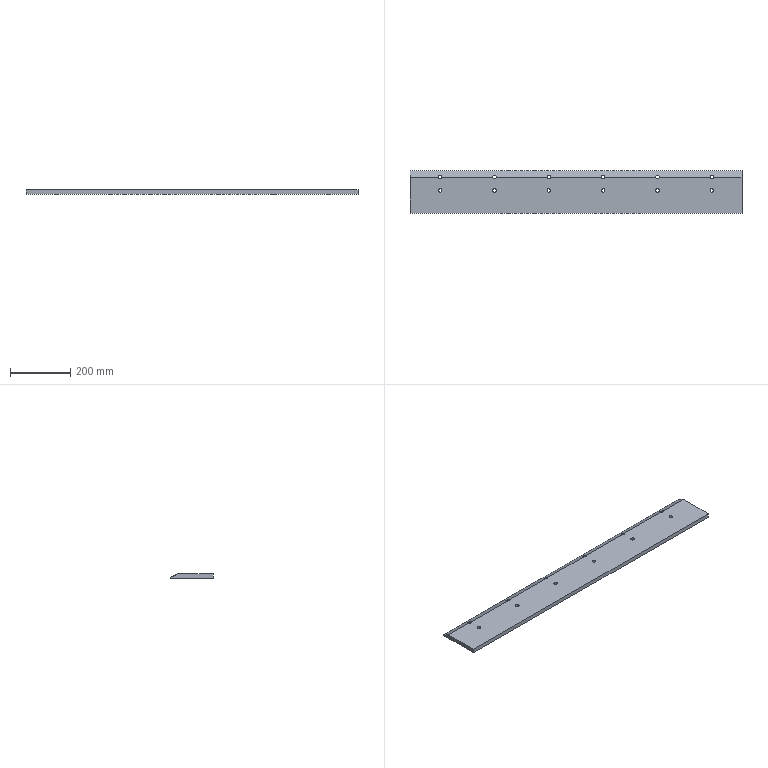Part | SolidWorks | features Chamfer 1, FlatPattern 1, SMBaseFlange 1, SheetMetal 1 | 1 solid | 31 faces | box 1100 x 140 x 14 mm | volume 1986347 mm3 | cylinder 24 | plane 7 | commonest cylinder face diameters 12 x24
STEP:
#1=CARTESIAN_POINT('',(1503.918,1234.342,-14.));
#2=VERTEX_POINT('',#1);
#3=CARTESIAN_POINT('',(1515.918,1234.342,-14.));
#4=VERTEX_POINT('',#3);
#5=CARTESIAN_POINT('',(1509.918,1234.342,-14.));
#6=DIRECTION('',(0.,0.,1.));
#7=DIRECTION('',(1.,0.,0.));
#8=AXIS2_PLACEMENT_3D('',#5,#6,#7);
#9=CIRCLE('',#8,6.);
#10=EDGE_CURVE('',#2,#4,#9,.T.);
#11=ORIENTED_EDGE('',*,*,#10,.F.);
#12=CARTESIAN_POINT('',(1503.918,1234.342,0.));
#13=VERTEX_POINT('',#12);
#14=CARTESIAN_POINT('',(1503.918,1234.342,-14.));
#15=DIRECTION('',(0.,0.,1.));
#16=VECTOR('',#15,1000.);
#17=LINE('',#14,#16);
#18=EDGE_CURVE('',#2,#13,#17,.T.);
#19=ORIENTED_EDGE('',*,*,#18,.T.);
#20=CARTESIAN_POINT('',(1515.918,1234.342,0.));
#21=VERTEX_POINT('',#20);
#22=CARTESIAN_POINT('',(1509.918,1234.342,0.));
#23=DIRECTION('',(0.,0.,1.));
#24=DIRECTION('',(1.,0.,0.));
#25=AXIS2_PLACEMENT_3D('',#22,#23,#24);
#26=CIRCLE('',#25,6.);
#27=EDGE_CURVE('',#13,#21,#26,.T.);
#28=ORIENTED_EDGE('',*,*,#27,.T.);
#29=CARTESIAN_POINT('',(1515.918,1234.342,-14.));
#30=DIRECTION('',(0.,0.,1.));
#31=VECTOR('',#30,1000.);
#32=LINE('',#29,#31);
#33=EDGE_CURVE('',#4,#21,#32,.T.);
#34=ORIENTED_EDGE('',*,*,#33,.F.);
#35=EDGE_LOOP('',(#11,#19,#28,#34));
#36=FACE_OUTER_BOUND('',#35,.T.);
#37=CARTESIAN_POINT('',(1509.918,1234.342,-14.));
#38=DIRECTION('',(0.,0.,1.));
#39=DIRECTION('',(1.,0.,0.));
#40=AXIS2_PLACEMENT_3D('',#37,#38,#39);
#41=CYLINDRICAL_SURFACE('',#40,6.);
#42=ADVANCED_FACE('',(#36),#41,.F.);
#43=CARTESIAN_POINT('',(1683.918,1234.342,-14.));
#44=VERTEX_POINT('',#43);
#45=CARTESIAN_POINT('',(1695.918,1234.342,-14.));
#46=VERTEX_POINT('',#45);
#47=CARTESIAN_POINT('',(1689.918,1234.342,-14.));
#48=DIRECTION('',(0.,0.,1.));
#49=DIRECTION('',(1.,0.,0.));
#50=AXIS2_PLACEMENT_3D('',#47,#48,#49);
#51=CIRCLE('',#50,6.);
#52=EDGE_CURVE('',#44,#46,#51,.T.);
#53=ORIENTED_EDGE('',*,*,#52,.F.);
#54=CARTESIAN_POINT('',(1683.918,1234.342,0.));
#55=VERTEX_POINT('',#54);
#56=CARTESIAN_POINT('',(1683.918,1234.342,-14.));
#57=DIRECTION('',(0.,0.,1.));
#58=VECTOR('',#57,1000.);
#59=LINE('',#56,#58);
#60=EDGE_CURVE('',#44,#55,#59,.T.);
#61=ORIENTED_EDGE('',*,*,#60,.T.);
#62=CARTESIAN_POINT('',(1695.918,1234.342,0.));
#63=VERTEX_POINT('',#62);
#64=CARTESIAN_POINT('',(1689.918,1234.342,0.));
#65=DIRECTION('',(0.,0.,1.));
#66=DIRECTION('',(1.,0.,0.));
#67=AXIS2_PLACEMENT_3D('',#64,#65,#66);
#68=CIRCLE('',#67,6.);
#69=EDGE_CURVE('',#55,#63,#68,.T.);
#70=ORIENTED_EDGE('',*,*,#69,.T.);
#71=CARTESIAN_POINT('',(1695.918,1234.342,-14.));
#72=DIRECTION('',(0.,0.,1.));
#73=VECTOR('',#72,1000.);
#74=LINE('',#71,#73);
#75=EDGE_CURVE('',#46,#63,#74,.T.);
#76=ORIENTED_EDGE('',*,*,#75,.F.);
#77=EDGE_LOOP('',(#53,#61,#70,#76));
#78=FACE_OUTER_BOUND('',#77,.T.);
#79=CARTESIAN_POINT('',(1689.918,1234.342,-14.));
#80=DIRECTION('',(0.,0.,1.));
#81=DIRECTION('',(1.,0.,0.));
#82=AXIS2_PLACEMENT_3D('',#79,#80,#81);
#83=CYLINDRICAL_SURFACE('',#82,6.);
#84=ADVANCED_FACE('',(#78),#83,.F.);
#85=CARTESIAN_POINT('',(1143.918,1234.342,-14.));
#86=VERTEX_POINT('',#85);
#87=CARTESIAN_POINT('',(1155.918,1234.342,-14.));
#88=VERTEX_POINT('',#87);
#89=CARTESIAN_POINT('',(1149.918,1234.342,-14.));
#90=DIRECTION('',(0.,0.,1.));
#91=DIRECTION('',(1.,0.,0.));
#92=AXIS2_PLACEMENT_3D('',#89,#90,#91);
#93=CIRCLE('',#92,6.);
#94=EDGE_CURVE('',#86,#88,#93,.T.);
#95=ORIENTED_EDGE('',*,*,#94,.F.);
#96=CARTESIAN_POINT('',(1143.918,1234.342,0.));
#97=VERTEX_POINT('',#96);
#98=CARTESIAN_POINT('',(1143.918,1234.342,-14.));
#99=DIRECTION('',(0.,0.,1.));
#100=VECTOR('',#99,1000.);
#101=LINE('',#98,#100);
#102=EDGE_CURVE('',#86,#97,#101,.T.);
#103=ORIENTED_EDGE('',*,*,#102,.T.);
#104=CARTESIAN_POINT('',(1155.918,1234.342,0.));
#105=VERTEX_POINT('',#104);
#106=CARTESIAN_POINT('',(1149.918,1234.342,0.));
#107=DIRECTION('',(0.,0.,1.));
#108=DIRECTION('',(1.,0.,0.));
#109=AXIS2_PLACEMENT_3D('',#106,#107,#108);
#110=CIRCLE('',#109,6.);
#111=EDGE_CURVE('',#97,#105,#110,.T.);
#112=ORIENTED_EDGE('',*,*,#111,.T.);
#113=CARTESIAN_POINT('',(1155.918,1234.342,-14.));
#114=DIRECTION('',(0.,0.,1.));
#115=VECTOR('',#114,1000.);
#116=LINE('',#113,#115);
#117=EDGE_CURVE('',#88,#105,#116,.T.);
#118=ORIENTED_EDGE('',*,*,#117,.F.);
#119=EDGE_LOOP('',(#95,#103,#112,#118));
#120=FACE_OUTER_BOUND('',#119,.T.);
#121=CARTESIAN_POINT('',(1149.918,1234.342,-14.));
#122=DIRECTION('',(0.,0.,1.));
#123=DIRECTION('',(1.,0.,0.));
#124=AXIS2_PLACEMENT_3D('',#121,#122,#123);
#125=CYLINDRICAL_SURFACE('',#124,6.);
#126=ADVANCED_FACE('',(#120),#125,.F.);
#127=CARTESIAN_POINT('',(1323.918,1234.342,-14.));
#128=VERTEX_POINT('',#127);
#129=CARTESIAN_POINT('',(1335.918,1234.342,-14.));
#130=VERTEX_POINT('',#129);
#131=CARTESIAN_POINT('',(1329.918,1234.342,-14.));
#132=DIRECTION('',(0.,0.,1.));
#133=DIRECTION('',(1.,0.,0.));
#134=AXIS2_PLACEMENT_3D('',#131,#132,#133);
#135=CIRCLE('',#134,6.);
#136=EDGE_CURVE('',#128,#130,#135,.T.);
#137=ORIENTED_EDGE('',*,*,#136,.F.);
#138=CARTESIAN_POINT('',(1323.918,1234.342,0.));
#139=VERTEX_POINT('',#138);
#140=CARTESIAN_POINT('',(1323.918,1234.342,-14.));
#141=DIRECTION('',(0.,0.,1.));
#142=VECTOR('',#141,1000.);
#143=LINE('',#140,#142);
#144=EDGE_CURVE('',#128,#139,#143,.T.);
#145=ORIENTED_EDGE('',*,*,#144,.T.);
#146=CARTESIAN_POINT('',(1335.918,1234.342,0.));
#147=VERTEX_POINT('',#146);
#148=CARTESIAN_POINT('',(1329.918,1234.342,0.));
#149=DIRECTION('',(0.,0.,1.));
#150=DIRECTION('',(1.,0.,0.));
#151=AXIS2_PLACEMENT_3D('',#148,#149,#150);
#152=CIRCLE('',#151,6.);
#153=EDGE_CURVE('',#139,#147,#152,.T.);
#154=ORIENTED_EDGE('',*,*,#153,.T.);
#155=CARTESIAN_POINT('',(1335.918,1234.342,-14.));
#156=DIRECTION('',(0.,0.,1.));
#157=VECTOR('',#156,1000.);
#158=LINE('',#155,#157);
#159=EDGE_CURVE('',#130,#147,#158,.T.);
#160=ORIENTED_EDGE('',*,*,#159,.F.);
#161=EDGE_LOOP('',(#137,#145,#154,#160));
#162=FACE_OUTER_BOUND('',#161,.T.);
#163=CARTESIAN_POINT('',(1329.918,1234.342,-14.));
#164=DIRECTION('',(0.,0.,1.));
#165=DIRECTION('',(1.,0.,0.));
#166=AXIS2_PLACEMENT_3D('',#163,#164,#165);
#167=CYLINDRICAL_SURFACE('',#166,6.);
#168=ADVANCED_FACE('',(#162),#167,.F.);
#169=CARTESIAN_POINT('',(2043.918,1234.342,-14.));
#170=VERTEX_POINT('',#169);
#171=CARTESIAN_POINT('',(2055.918,1234.342,-14.));
#172=VERTEX_POINT('',#171);
#173=CARTESIAN_POINT('',(2049.918,1234.342,-14.));
#174=DIRECTION('',(0.,0.,1.));
#175=DIRECTION('',(1.,0.,0.));
#176=AXIS2_PLACEMENT_3D('',#173,#174,#175);
#177=CIRCLE('',#176,6.);
#178=EDGE_CURVE('',#170,#172,#177,.T.);
#179=ORIENTED_EDGE('',*,*,#178,.F.);
#180=CARTESIAN_POINT('',(2043.918,1234.342,0.));
#181=VERTEX_POINT('',#180);
#182=CARTESIAN_POINT('',(2043.918,1234.342,-14.));
#183=DIRECTION('',(0.,0.,1.));
#184=VECTOR('',#183,1000.);
#185=LINE('',#182,#184);
#186=EDGE_CURVE('',#170,#181,#185,.T.);
#187=ORIENTED_EDGE('',*,*,#186,.T.);
#188=CARTESIAN_POINT('',(2055.918,1234.342,0.));
#189=VERTEX_POINT('',#188);
#190=CARTESIAN_POINT('',(2049.918,1234.342,0.));
#191=DIRECTION('',(0.,0.,1.));
#192=DIRECTION('',(1.,0.,0.));
#193=AXIS2_PLACEMENT_3D('',#190,#191,#192);
#194=CIRCLE('',#193,6.);
#195=EDGE_CURVE('',#181,#189,#194,.T.);
#196=ORIENTED_EDGE('',*,*,#195,.T.);
#197=CARTESIAN_POINT('',(2055.918,1234.342,-14.));
#198=DIRECTION('',(0.,0.,1.));
#199=VECTOR('',#198,1000.);
#200=LINE('',#197,#199);
#201=EDGE_CURVE('',#172,#189,#200,.T.);
#202=ORIENTED_EDGE('',*,*,#201,.F.);
#203=EDGE_LOOP('',(#179,#187,#196,#202));
#204=FACE_OUTER_BOUND('',#203,.T.);
#205=CARTESIAN_POINT('',(2049.918,1234.342,-14.));
#206=DIRECTION('',(0.,0.,1.));
#207=DIRECTION('',(1.,0.,0.));
#208=AXIS2_PLACEMENT_3D('',#205,#206,#207);
#209=CYLINDRICAL_SURFACE('',#208,6.);
#210=ADVANCED_FACE('',(#204),#209,.F.);
#211=CARTESIAN_POINT('',(1863.918,1234.342,-14.));
#212=VERTEX_POINT('',#211);
#213=CARTESIAN_POINT('',(1875.918,1234.342,-14.));
#214=VERTEX_POINT('',#213);
#215=CARTESIAN_POINT('',(1869.918,1234.342,-14.));
#216=DIRECTION('',(0.,0.,1.));
#217=DIRECTION('',(1.,0.,0.));
#218=AXIS2_PLACEMENT_3D('',#215,#216,#217);
#219=CIRCLE('',#218,6.);
#220=EDGE_CURVE('',#212,#214,#219,.T.);
#221=ORIENTED_EDGE('',*,*,#220,.F.);
#222=CARTESIAN_POINT('',(1863.918,1234.342,0.));
#223=VERTEX_POINT('',#222);
#224=CARTESIAN_POINT('',(1863.918,1234.342,-14.));
#225=DIRECTION('',(0.,0.,1.));
#226=VECTOR('',#225,1000.);
#227=LINE('',#224,#226);
#228=EDGE_CURVE('',#212,#223,#227,.T.);
#229=ORIENTED_EDGE('',*,*,#228,.T.);
#230=CARTESIAN_POINT('',(1875.918,1234.342,0.));
#231=VERTEX_POINT('',#230);
#232=CARTESIAN_POINT('',(1869.918,1234.342,0.));
#233=DIRECTION('',(0.,0.,1.));
#234=DIRECTION('',(1.,0.,0.));
#235=AXIS2_PLACEMENT_3D('',#232,#233,#234);
#236=CIRCLE('',#235,6.);
#237=EDGE_CURVE('',#223,#231,#236,.T.);
#238=ORIENTED_EDGE('',*,*,#237,.T.);
#239=CARTESIAN_POINT('',(1875.918,1234.342,-14.));
#240=DIRECTION('',(0.,0.,1.));
#241=VECTOR('',#240,1000.);
#242=LINE('',#239,#241);
#243=EDGE_CURVE('',#214,#231,#242,.T.);
#244=ORIENTED_EDGE('',*,*,#243,.F.);
#245=EDGE_LOOP('',(#221,#229,#238,#244));
#246=FACE_OUTER_BOUND('',#245,.T.);
#247=CARTESIAN_POINT('',(1869.918,1234.342,-14.));
#248=DIRECTION('',(0.,0.,1.));
#249=DIRECTION('',(1.,0.,0.));
#250=AXIS2_PLACEMENT_3D('',#247,#248,#249);
#251=CYLINDRICAL_SURFACE('',#250,6.);
#252=ADVANCED_FACE('',(#246),#251,.F.);
#253=CARTESIAN_POINT('',(1503.918,1279.342,-14.));
#254=VERTEX_POINT('',#253);
#255=CARTESIAN_POINT('',(1515.918,1279.342,-14.));
#256=VERTEX_POINT('',#255);
#257=CARTESIAN_POINT('',(1509.918,1279.342,-14.));
#258=DIRECTION('',(0.,0.,1.));
#259=DIRECTION('',(1.,0.,0.));
#260=AXIS2_PLACEMENT_3D('',#257,#258,#259);
#261=CIRCLE('',#260,6.);
#262=EDGE_CURVE('',#254,#256,#261,.T.);
#263=ORIENTED_EDGE('',*,*,#262,.F.);
#264=CARTESIAN_POINT('',(1503.918,1279.342,-1.565));
#265=VERTEX_POINT('',#264);
#266=CARTESIAN_POINT('',(1503.918,1279.342,-14.));
#267=DIRECTION('',(0.,0.,1.));
#268=VECTOR('',#267,1000.);
#269=LINE('',#266,#268);
#270=EDGE_CURVE('',#254,#265,#269,.T.);
#271=ORIENTED_EDGE('',*,*,#270,.T.);
#272=CARTESIAN_POINT('',(1504.721,1276.342,0.));
#273=VERTEX_POINT('',#272);
#274=CARTESIAN_POINT('',(1503.918,1279.342,-1.565));
#275=CARTESIAN_POINT('',(1503.918,1278.283,-1.013));
#276=CARTESIAN_POINT('',(1504.192,1277.259,-0.4787));
#277=CARTESIAN_POINT('',(1504.721,1276.342,0.));
#278=(BOUNDED_CURVE()B_SPLINE_CURVE(3,(#274,#275,#276,#277),.UNSPECIFIED.,.F.,.T.)B_SPLINE_CURVE_WITH_KNOTS((4,4),(4.712,5.236),.UNSPECIFIED.)CURVE()GEOMETRIC_REPRESENTATION_ITEM()RATIONAL_B_SPLINE_CURVE((1.,0.9773,0.9773,1.))REPRESENTATION_ITEM(''));
#279=EDGE_CURVE('',#265,#273,#278,.T.);
#280=ORIENTED_EDGE('',*,*,#279,.T.);
#281=CARTESIAN_POINT('',(1515.114,1276.342,0.));
#282=VERTEX_POINT('',#281);
#283=CARTESIAN_POINT('',(1509.918,1279.342,0.));
#284=DIRECTION('',(0.,0.,1.));
#285=DIRECTION('',(1.,0.,0.));
#286=AXIS2_PLACEMENT_3D('',#283,#284,#285);
#287=CIRCLE('',#286,6.);
#288=EDGE_CURVE('',#273,#282,#287,.T.);
#289=ORIENTED_EDGE('',*,*,#288,.T.);
#290=CARTESIAN_POINT('',(1515.918,1279.342,-1.565));
#291=VERTEX_POINT('',#290);
#292=CARTESIAN_POINT('',(1515.114,1276.342,0.));
#293=CARTESIAN_POINT('',(1515.643,1277.259,-0.4787));
#294=CARTESIAN_POINT('',(1515.918,1278.283,-1.013));
#295=CARTESIAN_POINT('',(1515.918,1279.342,-1.565));
#296=(BOUNDED_CURVE()B_SPLINE_CURVE(3,(#292,#293,#294,#295),.UNSPECIFIED.,.F.,.T.)B_SPLINE_CURVE_WITH_KNOTS((4,4),(1.047,1.571),.UNSPECIFIED.)CURVE()GEOMETRIC_REPRESENTATION_ITEM()RATIONAL_B_SPLINE_CURVE((1.,0.9773,0.9773,1.))REPRESENTATION_ITEM(''));
#297=EDGE_CURVE('',#282,#291,#296,.T.);
#298=ORIENTED_EDGE('',*,*,#297,.T.);
#299=CARTESIAN_POINT('',(1515.918,1279.342,-14.));
#300=DIRECTION('',(0.,0.,1.));
#301=VECTOR('',#300,1000.);
#302=LINE('',#299,#301);
#303=EDGE_CURVE('',#256,#291,#302,.T.);
#304=ORIENTED_EDGE('',*,*,#303,.F.);
#305=EDGE_LOOP('',(#263,#271,#280,#289,#298,#304));
#306=FACE_OUTER_BOUND('',#305,.T.);
#307=CARTESIAN_POINT('',(1509.918,1279.342,-14.));
#308=DIRECTION('',(0.,0.,1.));
#309=DIRECTION('',(1.,0.,0.));
#310=AXIS2_PLACEMENT_3D('',#307,#308,#309);
#311=CYLINDRICAL_SURFACE('',#310,6.);
#312=ADVANCED_FACE('',(#306),#311,.F.);
#313=CARTESIAN_POINT('',(1683.918,1279.342,-14.));
#314=VERTEX_POINT('',#313);
#315=CARTESIAN_POINT('',(1695.918,1279.342,-14.));
#316=VERTEX_POINT('',#315);
#317=CARTESIAN_POINT('',(1689.918,1279.342,-14.));
#318=DIRECTION('',(0.,0.,1.));
#319=DIRECTION('',(1.,0.,0.));
#320=AXIS2_PLACEMENT_3D('',#317,#318,#319);
#321=CIRCLE('',#320,6.);
#322=EDGE_CURVE('',#314,#316,#321,.T.);
#323=ORIENTED_EDGE('',*,*,#322,.F.);
#324=CARTESIAN_POINT('',(1683.918,1279.342,-1.565));
#325=VERTEX_POINT('',#324);
#326=CARTESIAN_POINT('',(1683.918,1279.342,-14.));
#327=DIRECTION('',(0.,0.,1.));
#328=VECTOR('',#327,1000.);
#329=LINE('',#326,#328);
#330=EDGE_CURVE('',#314,#325,#329,.T.);
#331=ORIENTED_EDGE('',*,*,#330,.T.);
#332=CARTESIAN_POINT('',(1684.721,1276.342,0.));
#333=VERTEX_POINT('',#332);
#334=CARTESIAN_POINT('',(1683.918,1279.342,-1.565));
#335=CARTESIAN_POINT('',(1683.918,1278.283,-1.013));
#336=CARTESIAN_POINT('',(1684.192,1277.259,-0.4787));
#337=CARTESIAN_POINT('',(1684.721,1276.342,0.));
#338=(BOUNDED_CURVE()B_SPLINE_CURVE(3,(#334,#335,#336,#337),.UNSPECIFIED.,.F.,.T.)B_SPLINE_CURVE_WITH_KNOTS((4,4),(4.712,5.236),.UNSPECIFIED.)CURVE()GEOMETRIC_REPRESENTATION_ITEM()RATIONAL_B_SPLINE_CURVE((1.,0.9773,0.9773,1.))REPRESENTATION_ITEM(''));
#339=EDGE_CURVE('',#325,#333,#338,.T.);
#340=ORIENTED_EDGE('',*,*,#339,.T.);
#341=CARTESIAN_POINT('',(1695.114,1276.342,0.));
#342=VERTEX_POINT('',#341);
#343=CARTESIAN_POINT('',(1689.918,1279.342,0.));
#344=DIRECTION('',(0.,0.,1.));
#345=DIRECTION('',(1.,0.,0.));
#346=AXIS2_PLACEMENT_3D('',#343,#344,#345);
#347=CIRCLE('',#346,6.);
#348=EDGE_CURVE('',#333,#342,#347,.T.);
#349=ORIENTED_EDGE('',*,*,#348,.T.);
#350=CARTESIAN_POINT('',(1695.918,1279.342,-1.565));
#351=VERTEX_POINT('',#350);
#352=CARTESIAN_POINT('',(1695.114,1276.342,0.));
#353=CARTESIAN_POINT('',(1695.643,1277.259,-0.4787));
#354=CARTESIAN_POINT('',(1695.918,1278.283,-1.013));
#355=CARTESIAN_POINT('',(1695.918,1279.342,-1.565));
#356=(BOUNDED_CURVE()B_SPLINE_CURVE(3,(#352,#353,#354,#355),.UNSPECIFIED.,.F.,.T.)B_SPLINE_CURVE_WITH_KNOTS((4,4),(1.047,1.571),.UNSPECIFIED.)CURVE()GEOMETRIC_REPRESENTATION_ITEM()RATIONAL_B_SPLINE_CURVE((1.,0.9773,0.9773,1.))REPRESENTATION_ITEM(''));
#357=EDGE_CURVE('',#342,#351,#356,.T.);
#358=ORIENTED_EDGE('',*,*,#357,.T.);
#359=CARTESIAN_POINT('',(1695.918,1279.342,-14.));
#360=DIRECTION('',(0.,0.,1.));
#361=VECTOR('',#360,1000.);
#362=LINE('',#359,#361);
#363=EDGE_CURVE('',#316,#351,#362,.T.);
#364=ORIENTED_EDGE('',*,*,#363,.F.);
#365=EDGE_LOOP('',(#323,#331,#340,#349,#358,#364));
#366=FACE_OUTER_BOUND('',#365,.T.);
#367=CARTESIAN_POINT('',(1689.918,1279.342,-14.));
#368=DIRECTION('',(0.,0.,1.));
#369=DIRECTION('',(1.,0.,0.));
#370=AXIS2_PLACEMENT_3D('',#367,#368,#369);
#371=CYLINDRICAL_SURFACE('',#370,6.);
#372=ADVANCED_FACE('',(#366),#371,.F.);
#373=CARTESIAN_POINT('',(1143.918,1279.342,-14.));
#374=VERTEX_POINT('',#373);
#375=CARTESIAN_POINT('',(1155.918,1279.342,-14.));
#376=VERTEX_POINT('',#375);
#377=CARTESIAN_POINT('',(1149.918,1279.342,-14.));
#378=DIRECTION('',(0.,0.,1.));
#379=DIRECTION('',(1.,0.,0.));
#380=AXIS2_PLACEMENT_3D('',#377,#378,#379);
#381=CIRCLE('',#380,6.);
#382=EDGE_CURVE('',#374,#376,#381,.T.);
#383=ORIENTED_EDGE('',*,*,#382,.F.);
#384=CARTESIAN_POINT('',(1143.918,1279.342,-1.565));
#385=VERTEX_POINT('',#384);
#386=CARTESIAN_POINT('',(1143.918,1279.342,-14.));
#387=DIRECTION('',(0.,0.,1.));
#388=VECTOR('',#387,1000.);
#389=LINE('',#386,#388);
#390=EDGE_CURVE('',#374,#385,#389,.T.);
#391=ORIENTED_EDGE('',*,*,#390,.T.);
#392=CARTESIAN_POINT('',(1144.721,1276.342,0.));
#393=VERTEX_POINT('',#392);
#394=CARTESIAN_POINT('',(1143.918,1279.342,-1.565));
#395=CARTESIAN_POINT('',(1143.918,1278.283,-1.013));
#396=CARTESIAN_POINT('',(1144.192,1277.259,-0.4787));
#397=CARTESIAN_POINT('',(1144.721,1276.342,0.));
#398=(BOUNDED_CURVE()B_SPLINE_CURVE(3,(#394,#395,#396,#397),.UNSPECIFIED.,.F.,.T.)B_SPLINE_CURVE_WITH_KNOTS((4,4),(4.712,5.236),.UNSPECIFIED.)CURVE()GEOMETRIC_REPRESENTATION_ITEM()RATIONAL_B_SPLINE_CURVE((1.,0.9773,0.9773,1.))REPRESENTATION_ITEM(''));
#399=EDGE_CURVE('',#385,#393,#398,.T.);
#400=ORIENTED_EDGE('',*,*,#399,.T.);
#401=CARTESIAN_POINT('',(1155.114,1276.342,0.));
#402=VERTEX_POINT('',#401);
#403=CARTESIAN_POINT('',(1149.918,1279.342,0.));
#404=DIRECTION('',(0.,0.,1.));
#405=DIRECTION('',(1.,0.,0.));
#406=AXIS2_PLACEMENT_3D('',#403,#404,#405);
#407=CIRCLE('',#406,6.);
#408=EDGE_CURVE('',#393,#402,#407,.T.);
#409=ORIENTED_EDGE('',*,*,#408,.T.);
#410=CARTESIAN_POINT('',(1155.918,1279.342,-1.565));
#411=VERTEX_POINT('',#410);
#412=CARTESIAN_POINT('',(1155.114,1276.342,0.));
#413=CARTESIAN_POINT('',(1155.643,1277.259,-0.4787));
#414=CARTESIAN_POINT('',(1155.918,1278.283,-1.013));
#415=CARTESIAN_POINT('',(1155.918,1279.342,-1.565));
#416=(BOUNDED_CURVE()B_SPLINE_CURVE(3,(#412,#413,#414,#415),.UNSPECIFIED.,.F.,.F.)B_SPLINE_CURVE_WITH_KNOTS((4,4),(1.047,1.571),.UNSPECIFIED.)CURVE()GEOMETRIC_REPRESENTATION_ITEM()RATIONAL_B_SPLINE_CURVE((1.,0.9773,0.9773,1.))REPRESENTATION_ITEM(''));
#417=EDGE_CURVE('',#402,#411,#416,.T.);
#418=ORIENTED_EDGE('',*,*,#417,.T.);
#419=CARTESIAN_POINT('',(1155.918,1279.342,-14.));
#420=DIRECTION('',(0.,0.,1.));
#421=VECTOR('',#420,1000.);
#422=LINE('',#419,#421);
#423=EDGE_CURVE('',#376,#411,#422,.T.);
#424=ORIENTED_EDGE('',*,*,#423,.F.);
#425=EDGE_LOOP('',(#383,#391,#400,#409,#418,#424));
#426=FACE_OUTER_BOUND('',#425,.T.);
#427=CARTESIAN_POINT('',(1149.918,1279.342,-14.));
#428=DIRECTION('',(0.,0.,1.));
#429=DIRECTION('',(1.,0.,0.));
#430=AXIS2_PLACEMENT_3D('',#427,#428,#429);
#431=CYLINDRICAL_SURFACE('',#430,6.);
#432=ADVANCED_FACE('',(#426),#431,.F.);
#433=CARTESIAN_POINT('',(1323.918,1279.342,-14.));
#434=VERTEX_POINT('',#433);
#435=CARTESIAN_POINT('',(1335.918,1279.342,-14.));
#436=VERTEX_POINT('',#435);
#437=CARTESIAN_POINT('',(1329.918,1279.342,-14.));
#438=DIRECTION('',(0.,0.,1.));
#439=DIRECTION('',(1.,0.,0.));
#440=AXIS2_PLACEMENT_3D('',#437,#438,#439);
#441=CIRCLE('',#440,6.);
#442=EDGE_CURVE('',#434,#436,#441,.T.);
#443=ORIENTED_EDGE('',*,*,#442,.F.);
#444=CARTESIAN_POINT('',(1323.918,1279.342,-1.565));
#445=VERTEX_POINT('',#444);
#446=CARTESIAN_POINT('',(1323.918,1279.342,-14.));
#447=DIRECTION('',(0.,0.,1.));
#448=VECTOR('',#447,1000.);
#449=LINE('',#446,#448);
#450=EDGE_CURVE('',#434,#445,#449,.T.);
#451=ORIENTED_EDGE('',*,*,#450,.T.);
#452=CARTESIAN_POINT('',(1324.721,1276.342,0.));
#453=VERTEX_POINT('',#452);
#454=CARTESIAN_POINT('',(1323.918,1279.342,-1.565));
#455=CARTESIAN_POINT('',(1323.918,1278.283,-1.013));
#456=CARTESIAN_POINT('',(1324.192,1277.259,-0.4787));
#457=CARTESIAN_POINT('',(1324.721,1276.342,0.));
#458=(BOUNDED_CURVE()B_SPLINE_CURVE(3,(#454,#455,#456,#457),.UNSPECIFIED.,.F.,.T.)B_SPLINE_CURVE_WITH_KNOTS((4,4),(4.712,5.236),.UNSPECIFIED.)CURVE()GEOMETRIC_REPRESENTATION_ITEM()RATIONAL_B_SPLINE_CURVE((1.,0.9773,0.9773,1.))REPRESENTATION_ITEM(''));
#459=EDGE_CURVE('',#445,#453,#458,.T.);
#460=ORIENTED_EDGE('',*,*,#459,.T.);
#461=CARTESIAN_POINT('',(1335.114,1276.342,0.));
#462=VERTEX_POINT('',#461);
#463=CARTESIAN_POINT('',(1329.918,1279.342,0.));
#464=DIRECTION('',(0.,0.,1.));
#465=DIRECTION('',(1.,0.,0.));
#466=AXIS2_PLACEMENT_3D('',#463,#464,#465);
#467=CIRCLE('',#466,6.);
#468=EDGE_CURVE('',#453,#462,#467,.T.);
#469=ORIENTED_EDGE('',*,*,#468,.T.);
#470=CARTESIAN_POINT('',(1335.918,1279.342,-1.565));
#471=VERTEX_POINT('',#470);
#472=CARTESIAN_POINT('',(1335.114,1276.342,0.));
#473=CARTESIAN_POINT('',(1335.643,1277.259,-0.4787));
#474=CARTESIAN_POINT('',(1335.918,1278.283,-1.013));
#475=CARTESIAN_POINT('',(1335.918,1279.342,-1.565));
#476=(BOUNDED_CURVE()B_SPLINE_CURVE(3,(#472,#473,#474,#475),.UNSPECIFIED.,.F.,.F.)B_SPLINE_CURVE_WITH_KNOTS((4,4),(1.047,1.571),.UNSPECIFIED.)CURVE()GEOMETRIC_REPRESENTATION_ITEM()RATIONAL_B_SPLINE_CURVE((1.,0.9773,0.9773,1.))REPRESENTATION_ITEM(''));
#477=EDGE_CURVE('',#462,#471,#476,.T.);
#478=ORIENTED_EDGE('',*,*,#477,.T.);
#479=CARTESIAN_POINT('',(1335.918,1279.342,-14.));
#480=DIRECTION('',(0.,0.,1.));
#481=VECTOR('',#480,1000.);
#482=LINE('',#479,#481);
#483=EDGE_CURVE('',#436,#471,#482,.T.);
#484=ORIENTED_EDGE('',*,*,#483,.F.);
#485=EDGE_LOOP('',(#443,#451,#460,#469,#478,#484));
#486=FACE_OUTER_BOUND('',#485,.T.);
#487=CARTESIAN_POINT('',(1329.918,1279.342,-14.));
#488=DIRECTION('',(0.,0.,1.));
#489=DIRECTION('',(1.,0.,0.));
#490=AXIS2_PLACEMENT_3D('',#487,#488,#489);
#491=CYLINDRICAL_SURFACE('',#490,6.);
#492=ADVANCED_FACE('',(#486),#491,.F.);
#493=CARTESIAN_POINT('',(2043.918,1279.342,-14.));
#494=VERTEX_POINT('',#493);
#495=CARTESIAN_POINT('',(2055.918,1279.342,-14.));
#496=VERTEX_POINT('',#495);
#497=CARTESIAN_POINT('',(2049.918,1279.342,-14.));
#498=DIRECTION('',(0.,0.,1.));
#499=DIRECTION('',(1.,0.,0.));
#500=AXIS2_PLACEMENT_3D('',#497,#498,#499);
#501=CIRCLE('',#500,6.);
#502=EDGE_CURVE('',#494,#496,#501,.T.);
#503=ORIENTED_EDGE('',*,*,#502,.F.);
#504=CARTESIAN_POINT('',(2043.918,1279.342,-1.565));
#505=VERTEX_POINT('',#504);
#506=CARTESIAN_POINT('',(2043.918,1279.342,-14.));
#507=DIRECTION('',(0.,0.,1.));
#508=VECTOR('',#507,1000.);
#509=LINE('',#506,#508);
#510=EDGE_CURVE('',#494,#505,#509,.T.);
#511=ORIENTED_EDGE('',*,*,#510,.T.);
#512=CARTESIAN_POINT('',(2044.721,1276.342,0.));
#513=VERTEX_POINT('',#512);
#514=CARTESIAN_POINT('',(2043.918,1279.342,-1.565));
#515=CARTESIAN_POINT('',(2043.918,1278.283,-1.013));
#516=CARTESIAN_POINT('',(2044.192,1277.259,-0.4787));
#517=CARTESIAN_POINT('',(2044.721,1276.342,0.));
#518=(BOUNDED_CURVE()B_SPLINE_CURVE(3,(#514,#515,#516,#517),.UNSPECIFIED.,.F.,.T.)B_SPLINE_CURVE_WITH_KNOTS((4,4),(4.712,5.236),.UNSPECIFIED.)CURVE()GEOMETRIC_REPRESENTATION_ITEM()RATIONAL_B_SPLINE_CURVE((1.,0.9773,0.9773,1.))REPRESENTATION_ITEM(''));
#519=EDGE_CURVE('',#505,#513,#518,.T.);
#520=ORIENTED_EDGE('',*,*,#519,.T.);
#521=CARTESIAN_POINT('',(2055.114,1276.342,0.));
#522=VERTEX_POINT('',#521);
#523=CARTESIAN_POINT('',(2049.918,1279.342,0.));
#524=DIRECTION('',(0.,0.,1.));
#525=DIRECTION('',(1.,0.,0.));
#526=AXIS2_PLACEMENT_3D('',#523,#524,#525);
#527=CIRCLE('',#526,6.);
#528=EDGE_CURVE('',#513,#522,#527,.T.);
#529=ORIENTED_EDGE('',*,*,#528,.T.);
#530=CARTESIAN_POINT('',(2055.918,1279.342,-1.565));
#531=VERTEX_POINT('',#530);
#532=CARTESIAN_POINT('',(2055.114,1276.342,0.));
#533=CARTESIAN_POINT('',(2055.643,1277.259,-0.4787));
#534=CARTESIAN_POINT('',(2055.918,1278.283,-1.013));
#535=CARTESIAN_POINT('',(2055.918,1279.342,-1.565));
#536=(BOUNDED_CURVE()B_SPLINE_CURVE(3,(#532,#533,#534,#535),.UNSPECIFIED.,.F.,.T.)B_SPLINE_CURVE_WITH_KNOTS((4,4),(1.047,1.571),.UNSPECIFIED.)CURVE()GEOMETRIC_REPRESENTATION_ITEM()RATIONAL_B_SPLINE_CURVE((1.,0.9773,0.9773,1.))REPRESENTATION_ITEM(''));
#537=EDGE_CURVE('',#522,#531,#536,.T.);
#538=ORIENTED_EDGE('',*,*,#537,.T.);
#539=CARTESIAN_POINT('',(2055.918,1279.342,-14.));
#540=DIRECTION('',(0.,0.,1.));
#541=VECTOR('',#540,1000.);
#542=LINE('',#539,#541);
#543=EDGE_CURVE('',#496,#531,#542,.T.);
#544=ORIENTED_EDGE('',*,*,#543,.F.);
#545=EDGE_LOOP('',(#503,#511,#520,#529,#538,#544));
#546=FACE_OUTER_BOUND('',#545,.T.);
#547=CARTESIAN_POINT('',(2049.918,1279.342,-14.));
#548=DIRECTION('',(0.,0.,1.));
#549=DIRECTION('',(1.,0.,0.));
#550=AXIS2_PLACEMENT_3D('',#547,#548,#549);
#551=CYLINDRICAL_SURFACE('',#550,6.);
#552=ADVANCED_FACE('',(#546),#551,.F.);
#553=CARTESIAN_POINT('',(1863.918,1279.342,-14.));
#554=VERTEX_POINT('',#553);
#555=CARTESIAN_POINT('',(1875.918,1279.342,-14.));
#556=VERTEX_POINT('',#555);
#557=CARTESIAN_POINT('',(1869.918,1279.342,-14.));
#558=DIRECTION('',(0.,0.,1.));
#559=DIRECTION('',(1.,0.,0.));
#560=AXIS2_PLACEMENT_3D('',#557,#558,#559);
#561=CIRCLE('',#560,6.);
#562=EDGE_CURVE('',#554,#556,#561,.T.);
#563=ORIENTED_EDGE('',*,*,#562,.F.);
#564=CARTESIAN_POINT('',(1863.918,1279.342,-1.565));
#565=VERTEX_POINT('',#564);
#566=CARTESIAN_POINT('',(1863.918,1279.342,-14.));
#567=DIRECTION('',(0.,0.,1.));
#568=VECTOR('',#567,1000.);
#569=LINE('',#566,#568);
#570=EDGE_CURVE('',#554,#565,#569,.T.);
#571=ORIENTED_EDGE('',*,*,#570,.T.);
#572=CARTESIAN_POINT('',(1864.721,1276.342,0.));
#573=VERTEX_POINT('',#572);
#574=CARTESIAN_POINT('',(1863.918,1279.342,-1.565));
#575=CARTESIAN_POINT('',(1863.918,1278.283,-1.013));
#576=CARTESIAN_POINT('',(1864.192,1277.259,-0.4787));
#577=CARTESIAN_POINT('',(1864.721,1276.342,0.));
#578=(BOUNDED_CURVE()B_SPLINE_CURVE(3,(#574,#575,#576,#577),.UNSPECIFIED.,.F.,.T.)B_SPLINE_CURVE_WITH_KNOTS((4,4),(4.712,5.236),.UNSPECIFIED.)CURVE()GEOMETRIC_REPRESENTATION_ITEM()RATIONAL_B_SPLINE_CURVE((1.,0.9773,0.9773,1.))REPRESENTATION_ITEM(''));
#579=EDGE_CURVE('',#565,#573,#578,.T.);
#580=ORIENTED_EDGE('',*,*,#579,.T.);
#581=CARTESIAN_POINT('',(1875.114,1276.342,0.));
#582=VERTEX_POINT('',#581);
#583=CARTESIAN_POINT('',(1869.918,1279.342,0.));
#584=DIRECTION('',(0.,0.,1.));
#585=DIRECTION('',(1.,0.,0.));
#586=AXIS2_PLACEMENT_3D('',#583,#584,#585);
#587=CIRCLE('',#586,6.);
#588=EDGE_CURVE('',#573,#582,#587,.T.);
#589=ORIENTED_EDGE('',*,*,#588,.T.);
#590=CARTESIAN_POINT('',(1875.918,1279.342,-1.565));
#591=VERTEX_POINT('',#590);
#592=CARTESIAN_POINT('',(1875.114,1276.342,0.));
#593=CARTESIAN_POINT('',(1875.643,1277.259,-0.4787));
#594=CARTESIAN_POINT('',(1875.918,1278.283,-1.013));
#595=CARTESIAN_POINT('',(1875.918,1279.342,-1.565));
#596=(BOUNDED_CURVE()B_SPLINE_CURVE(3,(#592,#593,#594,#595),.UNSPECIFIED.,.F.,.F.)B_SPLINE_CURVE_WITH_KNOTS((4,4),(1.047,1.571),.UNSPECIFIED.)CURVE()GEOMETRIC_REPRESENTATION_ITEM()RATIONAL_B_SPLINE_CURVE((1.,0.9773,0.9773,1.))REPRESENTATION_ITEM(''));
#597=EDGE_CURVE('',#582,#591,#596,.T.);
#598=ORIENTED_EDGE('',*,*,#597,.T.);
#599=CARTESIAN_POINT('',(1875.918,1279.342,-14.));
#600=DIRECTION('',(0.,0.,1.));
#601=VECTOR('',#600,1000.);
#602=LINE('',#599,#601);
#603=EDGE_CURVE('',#556,#591,#602,.T.);
#604=ORIENTED_EDGE('',*,*,#603,.F.);
#605=EDGE_LOOP('',(#563,#571,#580,#589,#598,#604));
#606=FACE_OUTER_BOUND('',#605,.T.);
#607=CARTESIAN_POINT('',(1869.918,1279.342,-14.));
#608=DIRECTION('',(0.,0.,1.));
#609=DIRECTION('',(1.,0.,0.));
#610=AXIS2_PLACEMENT_3D('',#607,#608,#609);
#611=CYLINDRICAL_SURFACE('',#610,6.);
#612=ADVANCED_FACE('',(#606),#611,.F.);
#613=CARTESIAN_POINT('',(1049.918,1299.342,-14.));
#614=VERTEX_POINT('',#613);
#615=CARTESIAN_POINT('',(1049.918,1299.342,-12.));
#616=VERTEX_POINT('',#615);
#617=CARTESIAN_POINT('',(1049.918,1299.342,-14.));
#618=DIRECTION('',(0.,0.,1.));
#619=VECTOR('',#618,1000.);
#620=LINE('',#617,#619);
#621=EDGE_CURVE('',#614,#616,#620,.T.);
#622=ORIENTED_EDGE('',*,*,#621,.T.);
#623=CARTESIAN_POINT('',(2149.918,1299.342,-12.));
#624=VERTEX_POINT('',#623);
#625=CARTESIAN_POINT('',(2149.918,1299.342,-12.));
#626=DIRECTION('',(1.,0.,0.));
#627=VECTOR('',#626,1000.);
#628=LINE('',#625,#627);
#629=EDGE_CURVE('',#616,#624,#628,.T.);
#630=ORIENTED_EDGE('',*,*,#629,.T.);
#631=CARTESIAN_POINT('',(2149.918,1299.342,-14.));
#632=VERTEX_POINT('',#631);
#633=CARTESIAN_POINT('',(2149.918,1299.342,-14.));
#634=DIRECTION('',(0.,0.,1.));
#635=VECTOR('',#634,1000.);
#636=LINE('',#633,#635);
#637=EDGE_CURVE('',#632,#624,#636,.T.);
#638=ORIENTED_EDGE('',*,*,#637,.F.);
#639=CARTESIAN_POINT('',(2149.918,1299.342,-14.));
#640=DIRECTION('',(-1.,0.,0.));
#641=VECTOR('',#640,1000.);
#642=LINE('',#639,#641);
#643=EDGE_CURVE('',#632,#614,#642,.T.);
#644=ORIENTED_EDGE('',*,*,#643,.T.);
#645=EDGE_LOOP('',(#622,#630,#638,#644));
#646=FACE_OUTER_BOUND('',#645,.T.);
#647=CARTESIAN_POINT('',(2149.918,1299.342,-14.));
#648=DIRECTION('',(0.,1.,0.));
#649=DIRECTION('',(-1.,0.,0.));
#650=AXIS2_PLACEMENT_3D('',#647,#648,#649);
#651=PLANE('',#650);
#652=ADVANCED_FACE('',(#646),#651,.T.);
#653=ORIENTED_EDGE('',*,*,#637,.T.);
#654=CARTESIAN_POINT('',(2149.918,1276.342,0.));
#655=VERTEX_POINT('',#654);
#656=CARTESIAN_POINT('',(2149.918,1190.118,44.987));
#657=DIRECTION('',(0.,-0.8866,0.4626));
#658=VECTOR('',#657,1000.);
#659=LINE('',#656,#658);
#660=EDGE_CURVE('',#624,#655,#659,.T.);
#661=ORIENTED_EDGE('',*,*,#660,.T.);
#662=CARTESIAN_POINT('',(2149.918,1159.342,0.));
#663=VERTEX_POINT('',#662);
#664=CARTESIAN_POINT('',(2149.918,1159.342,0.));
#665=DIRECTION('',(0.,1.,0.));
#666=VECTOR('',#665,1000.);
#667=LINE('',#664,#666);
#668=EDGE_CURVE('',#663,#655,#667,.T.);
#669=ORIENTED_EDGE('',*,*,#668,.F.);
#670=CARTESIAN_POINT('',(2149.918,1159.342,-14.));
#671=VERTEX_POINT('',#670);
#672=CARTESIAN_POINT('',(2149.918,1159.342,-14.));
#673=DIRECTION('',(0.,0.,1.));
#674=VECTOR('',#673,1000.);
#675=LINE('',#672,#674);
#676=EDGE_CURVE('',#671,#663,#675,.T.);
#677=ORIENTED_EDGE('',*,*,#676,.F.);
#678=CARTESIAN_POINT('',(2149.918,1159.342,-14.));
#679=DIRECTION('',(0.,1.,0.));
#680=VECTOR('',#679,1000.);
#681=LINE('',#678,#680);
#682=EDGE_CURVE('',#671,#632,#681,.T.);
#683=ORIENTED_EDGE('',*,*,#682,.T.);
#684=EDGE_LOOP('',(#653,#661,#669,#677,#683));
#685=FACE_OUTER_BOUND('',#684,.T.);
#686=CARTESIAN_POINT('',(2149.918,1159.342,-14.));
#687=DIRECTION('',(1.,0.,0.));
#688=DIRECTION('',(0.,0.,-1.));
#689=AXIS2_PLACEMENT_3D('',#686,#687,#688);
#690=PLANE('',#689);
#691=ADVANCED_FACE('',(#685),#690,.T.);
#692=CARTESIAN_POINT('',(1049.918,1159.342,0.));
#693=VERTEX_POINT('',#692);
#694=CARTESIAN_POINT('',(1049.918,1159.342,0.));
#695=DIRECTION('',(1.,0.,0.));
#696=VECTOR('',#695,1000.);
#697=LINE('',#694,#696);
#698=EDGE_CURVE('',#693,#663,#697,.T.);
#699=ORIENTED_EDGE('',*,*,#698,.F.);
#700=CARTESIAN_POINT('',(1049.918,1159.342,-14.));
#701=VERTEX_POINT('',#700);
#702=CARTESIAN_POINT('',(1049.918,1159.342,-14.));
#703=DIRECTION('',(0.,0.,1.));
#704=VECTOR('',#703,1000.);
#705=LINE('',#702,#704);
#706=EDGE_CURVE('',#701,#693,#705,.T.);
#707=ORIENTED_EDGE('',*,*,#706,.F.);
#708=CARTESIAN_POINT('',(1049.918,1159.342,-14.));
#709=DIRECTION('',(1.,0.,0.));
#710=VECTOR('',#709,1000.);
#711=LINE('',#708,#710);
#712=EDGE_CURVE('',#701,#671,#711,.T.);
#713=ORIENTED_EDGE('',*,*,#712,.T.);
#714=ORIENTED_EDGE('',*,*,#676,.T.);
#715=EDGE_LOOP('',(#699,#707,#713,#714));
#716=FACE_OUTER_BOUND('',#715,.T.);
#717=CARTESIAN_POINT('',(1049.918,1159.342,-14.));
#718=DIRECTION('',(0.,-1.,0.));
#719=DIRECTION('',(0.,0.,-1.));
#720=AXIS2_PLACEMENT_3D('',#717,#718,#719);
#721=PLANE('',#720);
#722=ADVANCED_FACE('',(#716),#721,.T.);
#723=CARTESIAN_POINT('',(1049.918,1276.342,0.));
#724=VERTEX_POINT('',#723);
#725=CARTESIAN_POINT('',(1049.918,1299.342,0.));
#726=DIRECTION('',(0.,-1.,0.));
#727=VECTOR('',#726,1000.);
#728=LINE('',#725,#727);
#729=EDGE_CURVE('',#724,#693,#728,.T.);
#730=ORIENTED_EDGE('',*,*,#729,.F.);
#731=CARTESIAN_POINT('',(1049.918,1300.162,-12.428));
#732=DIRECTION('',(0.,0.8866,-0.4626));
#733=VECTOR('',#732,1000.);
#734=LINE('',#731,#733);
#735=EDGE_CURVE('',#724,#616,#734,.T.);
#736=ORIENTED_EDGE('',*,*,#735,.T.);
#737=ORIENTED_EDGE('',*,*,#621,.F.);
#738=CARTESIAN_POINT('',(1049.918,1299.342,-14.));
#739=DIRECTION('',(0.,-1.,0.));
#740=VECTOR('',#739,1000.);
#741=LINE('',#738,#740);
#742=EDGE_CURVE('',#614,#701,#741,.T.);
#743=ORIENTED_EDGE('',*,*,#742,.T.);
#744=ORIENTED_EDGE('',*,*,#706,.T.);
#745=EDGE_LOOP('',(#730,#736,#737,#743,#744));
#746=FACE_OUTER_BOUND('',#745,.T.);
#747=CARTESIAN_POINT('',(1049.918,1299.342,-14.));
#748=DIRECTION('',(-1.,0.,0.));
#749=DIRECTION('',(0.,0.,1.));
#750=AXIS2_PLACEMENT_3D('',#747,#748,#749);
#751=PLANE('',#750);
#752=ADVANCED_FACE('',(#746),#751,.T.);
#753=CARTESIAN_POINT('',(1509.918,1234.342,-14.));
#754=DIRECTION('',(0.,0.,1.));
#755=DIRECTION('',(1.,0.,0.));
#756=AXIS2_PLACEMENT_3D('',#753,#754,#755);
#757=CIRCLE('',#756,6.);
#758=EDGE_CURVE('',#4,#2,#757,.T.);
#759=ORIENTED_EDGE('',*,*,#758,.T.);
#760=ORIENTED_EDGE('',*,*,#10,.T.);
#761=EDGE_LOOP('',(#759,#760));
#762=FACE_BOUND('',#761,.T.);
#763=CARTESIAN_POINT('',(1689.918,1234.342,-14.));
#764=DIRECTION('',(0.,0.,1.));
#765=DIRECTION('',(1.,0.,0.));
#766=AXIS2_PLACEMENT_3D('',#763,#764,#765);
#767=CIRCLE('',#766,6.);
#768=EDGE_CURVE('',#46,#44,#767,.T.);
#769=ORIENTED_EDGE('',*,*,#768,.T.);
#770=ORIENTED_EDGE('',*,*,#52,.T.);
#771=EDGE_LOOP('',(#769,#770));
#772=FACE_BOUND('',#771,.T.);
#773=CARTESIAN_POINT('',(1149.918,1234.342,-14.));
#774=DIRECTION('',(0.,0.,1.));
#775=DIRECTION('',(1.,0.,0.));
#776=AXIS2_PLACEMENT_3D('',#773,#774,#775);
#777=CIRCLE('',#776,6.);
#778=EDGE_CURVE('',#88,#86,#777,.T.);
#779=ORIENTED_EDGE('',*,*,#778,.T.);
#780=ORIENTED_EDGE('',*,*,#94,.T.);
#781=EDGE_LOOP('',(#779,#780));
#782=FACE_BOUND('',#781,.T.);
#783=CARTESIAN_POINT('',(1329.918,1234.342,-14.));
#784=DIRECTION('',(0.,0.,1.));
#785=DIRECTION('',(1.,0.,0.));
#786=AXIS2_PLACEMENT_3D('',#783,#784,#785);
#787=CIRCLE('',#786,6.);
#788=EDGE_CURVE('',#130,#128,#787,.T.);
#789=ORIENTED_EDGE('',*,*,#788,.T.);
#790=ORIENTED_EDGE('',*,*,#136,.T.);
#791=EDGE_LOOP('',(#789,#790));
#792=FACE_BOUND('',#791,.T.);
#793=CARTESIAN_POINT('',(2049.918,1234.342,-14.));
#794=DIRECTION('',(0.,0.,1.));
#795=DIRECTION('',(1.,0.,0.));
#796=AXIS2_PLACEMENT_3D('',#793,#794,#795);
#797=CIRCLE('',#796,6.);
#798=EDGE_CURVE('',#172,#170,#797,.T.);
#799=ORIENTED_EDGE('',*,*,#798,.T.);
#800=ORIENTED_EDGE('',*,*,#178,.T.);
#801=EDGE_LOOP('',(#799,#800));
#802=FACE_BOUND('',#801,.T.);
#803=CARTESIAN_POINT('',(1869.918,1234.342,-14.));
#804=DIRECTION('',(0.,0.,1.));
#805=DIRECTION('',(1.,0.,0.));
#806=AXIS2_PLACEMENT_3D('',#803,#804,#805);
#807=CIRCLE('',#806,6.);
#808=EDGE_CURVE('',#214,#212,#807,.T.);
#809=ORIENTED_EDGE('',*,*,#808,.T.);
#810=ORIENTED_EDGE('',*,*,#220,.T.);
#811=EDGE_LOOP('',(#809,#810));
#812=FACE_BOUND('',#811,.T.);
#813=CARTESIAN_POINT('',(1509.918,1279.342,-14.));
#814=DIRECTION('',(0.,0.,1.));
#815=DIRECTION('',(1.,0.,0.));
#816=AXIS2_PLACEMENT_3D('',#813,#814,#815);
#817=CIRCLE('',#816,6.);
#818=EDGE_CURVE('',#256,#254,#817,.T.);
#819=ORIENTED_EDGE('',*,*,#818,.T.);
#820=ORIENTED_EDGE('',*,*,#262,.T.);
#821=EDGE_LOOP('',(#819,#820));
#822=FACE_BOUND('',#821,.T.);
#823=CARTESIAN_POINT('',(1689.918,1279.342,-14.));
#824=DIRECTION('',(0.,0.,1.));
#825=DIRECTION('',(1.,0.,0.));
#826=AXIS2_PLACEMENT_3D('',#823,#824,#825);
#827=CIRCLE('',#826,6.);
#828=EDGE_CURVE('',#316,#314,#827,.T.);
#829=ORIENTED_EDGE('',*,*,#828,.T.);
#830=ORIENTED_EDGE('',*,*,#322,.T.);
#831=EDGE_LOOP('',(#829,#830));
#832=FACE_BOUND('',#831,.T.);
#833=CARTESIAN_POINT('',(1149.918,1279.342,-14.));
#834=DIRECTION('',(0.,0.,1.));
#835=DIRECTION('',(1.,0.,0.));
#836=AXIS2_PLACEMENT_3D('',#833,#834,#835);
#837=CIRCLE('',#836,6.);
#838=EDGE_CURVE('',#376,#374,#837,.T.);
#839=ORIENTED_EDGE('',*,*,#838,.T.);
#840=ORIENTED_EDGE('',*,*,#382,.T.);
#841=EDGE_LOOP('',(#839,#840));
#842=FACE_BOUND('',#841,.T.);
#843=CARTESIAN_POINT('',(1329.918,1279.342,-14.));
#844=DIRECTION('',(0.,0.,1.));
#845=DIRECTION('',(1.,0.,0.));
#846=AXIS2_PLACEMENT_3D('',#843,#844,#845);
#847=CIRCLE('',#846,6.);
#848=EDGE_CURVE('',#436,#434,#847,.T.);
#849=ORIENTED_EDGE('',*,*,#848,.T.);
#850=ORIENTED_EDGE('',*,*,#442,.T.);
#851=EDGE_LOOP('',(#849,#850));
#852=FACE_BOUND('',#851,.T.);
#853=CARTESIAN_POINT('',(2049.918,1279.342,-14.));
#854=DIRECTION('',(0.,0.,1.));
#855=DIRECTION('',(1.,0.,0.));
#856=AXIS2_PLACEMENT_3D('',#853,#854,#855);
#857=CIRCLE('',#856,6.);
#858=EDGE_CURVE('',#496,#494,#857,.T.);
#859=ORIENTED_EDGE('',*,*,#858,.T.);
#860=ORIENTED_EDGE('',*,*,#502,.T.);
#861=EDGE_LOOP('',(#859,#860));
#862=FACE_BOUND('',#861,.T.);
#863=CARTESIAN_POINT('',(1869.918,1279.342,-14.));
#864=DIRECTION('',(0.,0.,1.));
#865=DIRECTION('',(1.,0.,0.));
#866=AXIS2_PLACEMENT_3D('',#863,#864,#865);
#867=CIRCLE('',#866,6.);
#868=EDGE_CURVE('',#556,#554,#867,.T.);
#869=ORIENTED_EDGE('',*,*,#868,.T.);
#870=ORIENTED_EDGE('',*,*,#562,.T.);
#871=EDGE_LOOP('',(#869,#870));
#872=FACE_BOUND('',#871,.T.);
#873=ORIENTED_EDGE('',*,*,#643,.F.);
#874=ORIENTED_EDGE('',*,*,#682,.F.);
#875=ORIENTED_EDGE('',*,*,#712,.F.);
#876=ORIENTED_EDGE('',*,*,#742,.F.);
#877=EDGE_LOOP('',(#873,#874,#875,#876));
#878=FACE_OUTER_BOUND('',#877,.T.);
#879=CARTESIAN_POINT('',(0.,0.,-14.));
#880=DIRECTION('',(0.,0.,1.));
#881=DIRECTION('',(1.,0.,0.));
#882=AXIS2_PLACEMENT_3D('',#879,#880,#881);
#883=PLANE('',#882);
#884=ADVANCED_FACE('',(#762,#772,#782,#792,#802,#812,#822,#832,#842,#852,#862,#872,#878),#883,.F.);
#885=CARTESIAN_POINT('',(1509.918,1234.342,0.));
#886=DIRECTION('',(0.,0.,1.));
#887=DIRECTION('',(1.,0.,0.));
#888=AXIS2_PLACEMENT_3D('',#885,#886,#887);
#889=CIRCLE('',#888,6.);
#890=EDGE_CURVE('',#21,#13,#889,.T.);
#891=ORIENTED_EDGE('',*,*,#890,.F.);
#892=ORIENTED_EDGE('',*,*,#27,.F.);
#893=EDGE_LOOP('',(#891,#892));
#894=FACE_BOUND('',#893,.T.);
#895=CARTESIAN_POINT('',(1689.918,1234.342,0.));
#896=DIRECTION('',(0.,0.,1.));
#897=DIRECTION('',(1.,0.,0.));
#898=AXIS2_PLACEMENT_3D('',#895,#896,#897);
#899=CIRCLE('',#898,6.);
#900=EDGE_CURVE('',#63,#55,#899,.T.);
#901=ORIENTED_EDGE('',*,*,#900,.F.);
#902=ORIENTED_EDGE('',*,*,#69,.F.);
#903=EDGE_LOOP('',(#901,#902));
#904=FACE_BOUND('',#903,.T.);
#905=CARTESIAN_POINT('',(1149.918,1234.342,0.));
#906=DIRECTION('',(0.,0.,1.));
#907=DIRECTION('',(1.,0.,0.));
#908=AXIS2_PLACEMENT_3D('',#905,#906,#907);
#909=CIRCLE('',#908,6.);
#910=EDGE_CURVE('',#105,#97,#909,.T.);
#911=ORIENTED_EDGE('',*,*,#910,.F.);
#912=ORIENTED_EDGE('',*,*,#111,.F.);
#913=EDGE_LOOP('',(#911,#912));
#914=FACE_BOUND('',#913,.T.);
#915=CARTESIAN_POINT('',(1329.918,1234.342,0.));
#916=DIRECTION('',(0.,0.,1.));
#917=DIRECTION('',(1.,0.,0.));
#918=AXIS2_PLACEMENT_3D('',#915,#916,#917);
#919=CIRCLE('',#918,6.);
#920=EDGE_CURVE('',#147,#139,#919,.T.);
#921=ORIENTED_EDGE('',*,*,#920,.F.);
#922=ORIENTED_EDGE('',*,*,#153,.F.);
#923=EDGE_LOOP('',(#921,#922));
#924=FACE_BOUND('',#923,.T.);
#925=CARTESIAN_POINT('',(2049.918,1234.342,0.));
#926=DIRECTION('',(0.,0.,1.));
#927=DIRECTION('',(1.,0.,0.));
#928=AXIS2_PLACEMENT_3D('',#925,#926,#927);
#929=CIRCLE('',#928,6.);
#930=EDGE_CURVE('',#189,#181,#929,.T.);
#931=ORIENTED_EDGE('',*,*,#930,.F.);
#932=ORIENTED_EDGE('',*,*,#195,.F.);
#933=EDGE_LOOP('',(#931,#932));
#934=FACE_BOUND('',#933,.T.);
#935=CARTESIAN_POINT('',(1869.918,1234.342,0.));
#936=DIRECTION('',(0.,0.,1.));
#937=DIRECTION('',(1.,0.,0.));
#938=AXIS2_PLACEMENT_3D('',#935,#936,#937);
#939=CIRCLE('',#938,6.);
#940=EDGE_CURVE('',#231,#223,#939,.T.);
#941=ORIENTED_EDGE('',*,*,#940,.F.);
#942=ORIENTED_EDGE('',*,*,#237,.F.);
#943=EDGE_LOOP('',(#941,#942));
#944=FACE_BOUND('',#943,.T.);
#945=ORIENTED_EDGE('',*,*,#668,.T.);
#946=CARTESIAN_POINT('',(0.,1276.342,0.));
#947=DIRECTION('',(-1.,0.,0.));
#948=VECTOR('',#947,1000.);
#949=LINE('',#946,#948);
#950=EDGE_CURVE('',#655,#522,#949,.T.);
#951=ORIENTED_EDGE('',*,*,#950,.T.);
#952=ORIENTED_EDGE('',*,*,#528,.F.);
#953=CARTESIAN_POINT('',(0.,1276.342,0.));
#954=DIRECTION('',(-1.,0.,0.));
#955=VECTOR('',#954,1000.);
#956=LINE('',#953,#955);
#957=EDGE_CURVE('',#513,#582,#956,.T.);
#958=ORIENTED_EDGE('',*,*,#957,.T.);
#959=ORIENTED_EDGE('',*,*,#588,.F.);
#960=CARTESIAN_POINT('',(0.,1276.342,0.));
#961=DIRECTION('',(-1.,0.,0.));
#962=VECTOR('',#961,1000.);
#963=LINE('',#960,#962);
#964=EDGE_CURVE('',#573,#342,#963,.T.);
#965=ORIENTED_EDGE('',*,*,#964,.T.);
#966=ORIENTED_EDGE('',*,*,#348,.F.);
#967=CARTESIAN_POINT('',(0.,1276.342,0.));
#968=DIRECTION('',(-1.,0.,0.));
#969=VECTOR('',#968,1000.);
#970=LINE('',#967,#969);
#971=EDGE_CURVE('',#333,#282,#970,.T.);
#972=ORIENTED_EDGE('',*,*,#971,.T.);
#973=ORIENTED_EDGE('',*,*,#288,.F.);
#974=CARTESIAN_POINT('',(0.,1276.342,0.));
#975=DIRECTION('',(-1.,0.,0.));
#976=VECTOR('',#975,1000.);
#977=LINE('',#974,#976);
#978=EDGE_CURVE('',#273,#462,#977,.T.);
#979=ORIENTED_EDGE('',*,*,#978,.T.);
#980=ORIENTED_EDGE('',*,*,#468,.F.);
#981=CARTESIAN_POINT('',(0.,1276.342,0.));
#982=DIRECTION('',(-1.,0.,0.));
#983=VECTOR('',#982,1000.);
#984=LINE('',#981,#983);
#985=EDGE_CURVE('',#453,#402,#984,.T.);
#986=ORIENTED_EDGE('',*,*,#985,.T.);
#987=ORIENTED_EDGE('',*,*,#408,.F.);
#988=CARTESIAN_POINT('',(0.,1276.342,0.));
#989=DIRECTION('',(-1.,0.,0.));
#990=VECTOR('',#989,1000.);
#991=LINE('',#988,#990);
#992=EDGE_CURVE('',#393,#724,#991,.T.);
#993=ORIENTED_EDGE('',*,*,#992,.T.);
#994=ORIENTED_EDGE('',*,*,#729,.T.);
#995=ORIENTED_EDGE('',*,*,#698,.T.);
#996=EDGE_LOOP('',(#945,#951,#952,#958,#959,#965,#966,#972,#973,#979,#980,#986,#987,#993,#994,#995));
#997=FACE_OUTER_BOUND('',#996,.T.);
#998=CARTESIAN_POINT('',(0.,0.,0.));
#999=DIRECTION('',(0.,0.,1.));
#1000=DIRECTION('',(1.,0.,0.));
#1001=AXIS2_PLACEMENT_3D('',#998,#999,#1000);
#1002=PLANE('',#1001);
#1003=ADVANCED_FACE('',(#894,#904,#914,#924,#934,#944,#997),#1002,.T.);
#1004=ORIENTED_EDGE('',*,*,#570,.F.);
#1005=ORIENTED_EDGE('',*,*,#868,.F.);
#1006=ORIENTED_EDGE('',*,*,#603,.T.);
#1007=CARTESIAN_POINT('',(1875.918,1279.342,-1.565));
#1008=CARTESIAN_POINT('',(1875.918,1291.342,-7.826));
#1009=CARTESIAN_POINT('',(1863.918,1291.342,-7.826));
#1010=CARTESIAN_POINT('',(1863.918,1279.342,-1.565));
#1011=(BOUNDED_CURVE()B_SPLINE_CURVE(3,(#1007,#1008,#1009,#1010),.UNSPECIFIED.,.F.,.F.)B_SPLINE_CURVE_WITH_KNOTS((4,4),(1.571,4.712),.UNSPECIFIED.)CURVE()GEOMETRIC_REPRESENTATION_ITEM()RATIONAL_B_SPLINE_CURVE((1.,0.3333,0.3333,1.))REPRESENTATION_ITEM(''));
#1012=EDGE_CURVE('',#591,#565,#1011,.T.);
#1013=ORIENTED_EDGE('',*,*,#1012,.T.);
#1014=EDGE_LOOP('',(#1004,#1005,#1006,#1013));
#1015=FACE_OUTER_BOUND('',#1014,.T.);
#1016=CARTESIAN_POINT('',(1869.918,1279.342,-14.));
#1017=DIRECTION('',(0.,0.,1.));
#1018=DIRECTION('',(1.,0.,0.));
#1019=AXIS2_PLACEMENT_3D('',#1016,#1017,#1018);
#1020=CYLINDRICAL_SURFACE('',#1019,6.);
#1021=ADVANCED_FACE('',(#1015),#1020,.F.);
#1022=ORIENTED_EDGE('',*,*,#510,.F.);
#1023=ORIENTED_EDGE('',*,*,#858,.F.);
#1024=ORIENTED_EDGE('',*,*,#543,.T.);
#1025=CARTESIAN_POINT('',(2055.918,1279.342,-1.565));
#1026=CARTESIAN_POINT('',(2055.918,1291.342,-7.826));
#1027=CARTESIAN_POINT('',(2043.918,1291.342,-7.826));
#1028=CARTESIAN_POINT('',(2043.918,1279.342,-1.565));
#1029=(BOUNDED_CURVE()B_SPLINE_CURVE(3,(#1025,#1026,#1027,#1028),.UNSPECIFIED.,.F.,.T.)B_SPLINE_CURVE_WITH_KNOTS((4,4),(1.571,4.712),.UNSPECIFIED.)CURVE()GEOMETRIC_REPRESENTATION_ITEM()RATIONAL_B_SPLINE_CURVE((1.,0.3333,0.3333,1.))REPRESENTATION_ITEM(''));
#1030=EDGE_CURVE('',#531,#505,#1029,.T.);
#1031=ORIENTED_EDGE('',*,*,#1030,.T.);
#1032=EDGE_LOOP('',(#1022,#1023,#1024,#1031));
#1033=FACE_OUTER_BOUND('',#1032,.T.);
#1034=CARTESIAN_POINT('',(2049.918,1279.342,-14.));
#1035=DIRECTION('',(0.,0.,1.));
#1036=DIRECTION('',(1.,0.,0.));
#1037=AXIS2_PLACEMENT_3D('',#1034,#1035,#1036);
#1038=CYLINDRICAL_SURFACE('',#1037,6.);
#1039=ADVANCED_FACE('',(#1033),#1038,.F.);
#1040=ORIENTED_EDGE('',*,*,#450,.F.);
#1041=ORIENTED_EDGE('',*,*,#848,.F.);
#1042=ORIENTED_EDGE('',*,*,#483,.T.);
#1043=CARTESIAN_POINT('',(1335.918,1279.342,-1.565));
#1044=CARTESIAN_POINT('',(1335.918,1291.342,-7.826));
#1045=CARTESIAN_POINT('',(1323.918,1291.342,-7.826));
#1046=CARTESIAN_POINT('',(1323.918,1279.342,-1.565));
#1047=(BOUNDED_CURVE()B_SPLINE_CURVE(3,(#1043,#1044,#1045,#1046),.UNSPECIFIED.,.F.,.T.)B_SPLINE_CURVE_WITH_KNOTS((4,4),(1.571,4.712),.UNSPECIFIED.)CURVE()GEOMETRIC_REPRESENTATION_ITEM()RATIONAL_B_SPLINE_CURVE((1.,0.3333,0.3333,1.))REPRESENTATION_ITEM(''));
#1048=EDGE_CURVE('',#471,#445,#1047,.T.);
#1049=ORIENTED_EDGE('',*,*,#1048,.T.);
#1050=EDGE_LOOP('',(#1040,#1041,#1042,#1049));
#1051=FACE_OUTER_BOUND('',#1050,.T.);
#1052=CARTESIAN_POINT('',(1329.918,1279.342,-14.));
#1053=DIRECTION('',(0.,0.,1.));
#1054=DIRECTION('',(1.,0.,0.));
#1055=AXIS2_PLACEMENT_3D('',#1052,#1053,#1054);
#1056=CYLINDRICAL_SURFACE('',#1055,6.);
#1057=ADVANCED_FACE('',(#1051),#1056,.F.);
#1058=ORIENTED_EDGE('',*,*,#390,.F.);
#1059=ORIENTED_EDGE('',*,*,#838,.F.);
#1060=ORIENTED_EDGE('',*,*,#423,.T.);
#1061=CARTESIAN_POINT('',(1155.918,1279.342,-1.565));
#1062=CARTESIAN_POINT('',(1155.918,1291.342,-7.826));
#1063=CARTESIAN_POINT('',(1143.918,1291.342,-7.826));
#1064=CARTESIAN_POINT('',(1143.918,1279.342,-1.565));
#1065=(BOUNDED_CURVE()B_SPLINE_CURVE(3,(#1061,#1062,#1063,#1064),.UNSPECIFIED.,.F.,.T.)B_SPLINE_CURVE_WITH_KNOTS((4,4),(1.571,4.712),.UNSPECIFIED.)CURVE()GEOMETRIC_REPRESENTATION_ITEM()RATIONAL_B_SPLINE_CURVE((1.,0.3333,0.3333,1.))REPRESENTATION_ITEM(''));
#1066=EDGE_CURVE('',#411,#385,#1065,.T.);
#1067=ORIENTED_EDGE('',*,*,#1066,.T.);
#1068=EDGE_LOOP('',(#1058,#1059,#1060,#1067));
#1069=FACE_OUTER_BOUND('',#1068,.T.);
#1070=CARTESIAN_POINT('',(1149.918,1279.342,-14.));
#1071=DIRECTION('',(0.,0.,1.));
#1072=DIRECTION('',(1.,0.,0.));
#1073=AXIS2_PLACEMENT_3D('',#1070,#1071,#1072);
#1074=CYLINDRICAL_SURFACE('',#1073,6.);
#1075=ADVANCED_FACE('',(#1069),#1074,.F.);
#1076=ORIENTED_EDGE('',*,*,#330,.F.);
#1077=ORIENTED_EDGE('',*,*,#828,.F.);
#1078=ORIENTED_EDGE('',*,*,#363,.T.);
#1079=CARTESIAN_POINT('',(1695.918,1279.342,-1.565));
#1080=CARTESIAN_POINT('',(1695.918,1291.342,-7.826));
#1081=CARTESIAN_POINT('',(1683.918,1291.342,-7.826));
#1082=CARTESIAN_POINT('',(1683.918,1279.342,-1.565));
#1083=(BOUNDED_CURVE()B_SPLINE_CURVE(3,(#1079,#1080,#1081,#1082),.UNSPECIFIED.,.F.,.T.)B_SPLINE_CURVE_WITH_KNOTS((4,4),(1.571,4.712),.UNSPECIFIED.)CURVE()GEOMETRIC_REPRESENTATION_ITEM()RATIONAL_B_SPLINE_CURVE((1.,0.3333,0.3333,1.))REPRESENTATION_ITEM(''));
#1084=EDGE_CURVE('',#351,#325,#1083,.T.);
#1085=ORIENTED_EDGE('',*,*,#1084,.T.);
#1086=EDGE_LOOP('',(#1076,#1077,#1078,#1085));
#1087=FACE_OUTER_BOUND('',#1086,.T.);
#1088=CARTESIAN_POINT('',(1689.918,1279.342,-14.));
#1089=DIRECTION('',(0.,0.,1.));
#1090=DIRECTION('',(1.,0.,0.));
#1091=AXIS2_PLACEMENT_3D('',#1088,#1089,#1090);
#1092=CYLINDRICAL_SURFACE('',#1091,6.);
#1093=ADVANCED_FACE('',(#1087),#1092,.F.);
#1094=ORIENTED_EDGE('',*,*,#270,.F.);
#1095=ORIENTED_EDGE('',*,*,#818,.F.);
#1096=ORIENTED_EDGE('',*,*,#303,.T.);
#1097=CARTESIAN_POINT('',(1515.918,1279.342,-1.565));
#1098=CARTESIAN_POINT('',(1515.918,1291.342,-7.826));
#1099=CARTESIAN_POINT('',(1503.918,1291.342,-7.826));
#1100=CARTESIAN_POINT('',(1503.918,1279.342,-1.565));
#1101=(BOUNDED_CURVE()B_SPLINE_CURVE(3,(#1097,#1098,#1099,#1100),.UNSPECIFIED.,.F.,.F.)B_SPLINE_CURVE_WITH_KNOTS((4,4),(1.571,4.712),.UNSPECIFIED.)CURVE()GEOMETRIC_REPRESENTATION_ITEM()RATIONAL_B_SPLINE_CURVE((1.,0.3333,0.3333,1.))REPRESENTATION_ITEM(''));
#1102=EDGE_CURVE('',#291,#265,#1101,.T.);
#1103=ORIENTED_EDGE('',*,*,#1102,.T.);
#1104=EDGE_LOOP('',(#1094,#1095,#1096,#1103));
#1105=FACE_OUTER_BOUND('',#1104,.T.);
#1106=CARTESIAN_POINT('',(1509.918,1279.342,-14.));
#1107=DIRECTION('',(0.,0.,1.));
#1108=DIRECTION('',(1.,0.,0.));
#1109=AXIS2_PLACEMENT_3D('',#1106,#1107,#1108);
#1110=CYLINDRICAL_SURFACE('',#1109,6.);
#1111=ADVANCED_FACE('',(#1105),#1110,.F.);
#1112=ORIENTED_EDGE('',*,*,#228,.F.);
#1113=ORIENTED_EDGE('',*,*,#808,.F.);
#1114=ORIENTED_EDGE('',*,*,#243,.T.);
#1115=ORIENTED_EDGE('',*,*,#940,.T.);
#1116=EDGE_LOOP('',(#1112,#1113,#1114,#1115));
#1117=FACE_OUTER_BOUND('',#1116,.T.);
#1118=CARTESIAN_POINT('',(1869.918,1234.342,-14.));
#1119=DIRECTION('',(0.,0.,1.));
#1120=DIRECTION('',(1.,0.,0.));
#1121=AXIS2_PLACEMENT_3D('',#1118,#1119,#1120);
#1122=CYLINDRICAL_SURFACE('',#1121,6.);
#1123=ADVANCED_FACE('',(#1117),#1122,.F.);
#1124=ORIENTED_EDGE('',*,*,#186,.F.);
#1125=ORIENTED_EDGE('',*,*,#798,.F.);
#1126=ORIENTED_EDGE('',*,*,#201,.T.);
#1127=ORIENTED_EDGE('',*,*,#930,.T.);
#1128=EDGE_LOOP('',(#1124,#1125,#1126,#1127));
#1129=FACE_OUTER_BOUND('',#1128,.T.);
#1130=CARTESIAN_POINT('',(2049.918,1234.342,-14.));
#1131=DIRECTION('',(0.,0.,1.));
#1132=DIRECTION('',(1.,0.,0.));
#1133=AXIS2_PLACEMENT_3D('',#1130,#1131,#1132);
#1134=CYLINDRICAL_SURFACE('',#1133,6.);
#1135=ADVANCED_FACE('',(#1129),#1134,.F.);
#1136=ORIENTED_EDGE('',*,*,#144,.F.);
#1137=ORIENTED_EDGE('',*,*,#788,.F.);
#1138=ORIENTED_EDGE('',*,*,#159,.T.);
#1139=ORIENTED_EDGE('',*,*,#920,.T.);
#1140=EDGE_LOOP('',(#1136,#1137,#1138,#1139));
#1141=FACE_OUTER_BOUND('',#1140,.T.);
#1142=CARTESIAN_POINT('',(1329.918,1234.342,-14.));
#1143=DIRECTION('',(0.,0.,1.));
#1144=DIRECTION('',(1.,0.,0.));
#1145=AXIS2_PLACEMENT_3D('',#1142,#1143,#1144);
#1146=CYLINDRICAL_SURFACE('',#1145,6.);
#1147=ADVANCED_FACE('',(#1141),#1146,.F.);
#1148=ORIENTED_EDGE('',*,*,#102,.F.);
#1149=ORIENTED_EDGE('',*,*,#778,.F.);
#1150=ORIENTED_EDGE('',*,*,#117,.T.);
#1151=ORIENTED_EDGE('',*,*,#910,.T.);
#1152=EDGE_LOOP('',(#1148,#1149,#1150,#1151));
#1153=FACE_OUTER_BOUND('',#1152,.T.);
#1154=CARTESIAN_POINT('',(1149.918,1234.342,-14.));
#1155=DIRECTION('',(0.,0.,1.));
#1156=DIRECTION('',(1.,0.,0.));
#1157=AXIS2_PLACEMENT_3D('',#1154,#1155,#1156);
#1158=CYLINDRICAL_SURFACE('',#1157,6.);
#1159=ADVANCED_FACE('',(#1153),#1158,.F.);
#1160=ORIENTED_EDGE('',*,*,#60,.F.);
#1161=ORIENTED_EDGE('',*,*,#768,.F.);
#1162=ORIENTED_EDGE('',*,*,#75,.T.);
#1163=ORIENTED_EDGE('',*,*,#900,.T.);
#1164=EDGE_LOOP('',(#1160,#1161,#1162,#1163));
#1165=FACE_OUTER_BOUND('',#1164,.T.);
#1166=CARTESIAN_POINT('',(1689.918,1234.342,-14.));
#1167=DIRECTION('',(0.,0.,1.));
#1168=DIRECTION('',(1.,0.,0.));
#1169=AXIS2_PLACEMENT_3D('',#1166,#1167,#1168);
#1170=CYLINDRICAL_SURFACE('',#1169,6.);
#1171=ADVANCED_FACE('',(#1165),#1170,.F.);
#1172=ORIENTED_EDGE('',*,*,#18,.F.);
#1173=ORIENTED_EDGE('',*,*,#758,.F.);
#1174=ORIENTED_EDGE('',*,*,#33,.T.);
#1175=ORIENTED_EDGE('',*,*,#890,.T.);
#1176=EDGE_LOOP('',(#1172,#1173,#1174,#1175));
#1177=FACE_OUTER_BOUND('',#1176,.T.);
#1178=CARTESIAN_POINT('',(1509.918,1234.342,-14.));
#1179=DIRECTION('',(0.,0.,1.));
#1180=DIRECTION('',(1.,0.,0.));
#1181=AXIS2_PLACEMENT_3D('',#1178,#1179,#1180);
#1182=CYLINDRICAL_SURFACE('',#1181,6.);
#1183=ADVANCED_FACE('',(#1177),#1182,.F.);
#1184=ORIENTED_EDGE('',*,*,#660,.F.);
#1185=ORIENTED_EDGE('',*,*,#629,.F.);
#1186=ORIENTED_EDGE('',*,*,#735,.F.);
#1187=ORIENTED_EDGE('',*,*,#992,.F.);
#1188=ORIENTED_EDGE('',*,*,#399,.F.);
#1189=ORIENTED_EDGE('',*,*,#1066,.F.);
#1190=ORIENTED_EDGE('',*,*,#417,.F.);
#1191=ORIENTED_EDGE('',*,*,#985,.F.);
#1192=ORIENTED_EDGE('',*,*,#459,.F.);
#1193=ORIENTED_EDGE('',*,*,#1048,.F.);
#1194=ORIENTED_EDGE('',*,*,#477,.F.);
#1195=ORIENTED_EDGE('',*,*,#978,.F.);
#1196=ORIENTED_EDGE('',*,*,#279,.F.);
#1197=ORIENTED_EDGE('',*,*,#1102,.F.);
#1198=ORIENTED_EDGE('',*,*,#297,.F.);
#1199=ORIENTED_EDGE('',*,*,#971,.F.);
#1200=ORIENTED_EDGE('',*,*,#339,.F.);
#1201=ORIENTED_EDGE('',*,*,#1084,.F.);
#1202=ORIENTED_EDGE('',*,*,#357,.F.);
#1203=ORIENTED_EDGE('',*,*,#964,.F.);
#1204=ORIENTED_EDGE('',*,*,#579,.F.);
#1205=ORIENTED_EDGE('',*,*,#1012,.F.);
#1206=ORIENTED_EDGE('',*,*,#597,.F.);
#1207=ORIENTED_EDGE('',*,*,#957,.F.);
#1208=ORIENTED_EDGE('',*,*,#519,.F.);
#1209=ORIENTED_EDGE('',*,*,#1030,.F.);
#1210=ORIENTED_EDGE('',*,*,#537,.F.);
#1211=ORIENTED_EDGE('',*,*,#950,.F.);
#1212=EDGE_LOOP('',(#1184,#1185,#1186,#1187,#1188,#1189,#1190,#1191,#1192,#1193,#1194,#1195,#1196,#1197,#1198,#1199,#1200,#1201,#1202,#1203,#1204,#1205,#1206,#1207,#1208,#1209,#1210,#1211));
#1213=FACE_OUTER_BOUND('',#1212,.T.);
#1214=CARTESIAN_POINT('',(0.,1276.342,0.));
#1215=DIRECTION('',(0.,-0.4626,-0.8866));
#1216=DIRECTION('',(-1.,0.,0.));
#1217=AXIS2_PLACEMENT_3D('',#1214,#1215,#1216);
#1218=PLANE('',#1217);
#1219=ADVANCED_FACE('',(#1213),#1218,.F.);
#1220=CLOSED_SHELL('',(#42,#84,#126,#168,#210,#252,#312,#372,#432,#492,#552,#612,#652,#691,#722,#752,#884,#1003,#1021,#1039,#1057,#1075,#1093,#1111,#1123,#1135,#1147,#1159,#1171,#1183,#1219));
#1221=MANIFOLD_SOLID_BREP('',#1220);
#1222=CARTESIAN_POINT('',(0.,0.,0.));
#1223=DIRECTION('',(0.,0.,1.));
#1224=DIRECTION('',(1.,0.,0.));
#1225=AXIS2_PLACEMENT_3D('',#1222,#1223,#1224);
#1226=(LENGTH_UNIT()NAMED_UNIT(*)SI_UNIT(.MILLI.,.METRE.));
#1227=UNCERTAINTY_MEASURE_WITH_UNIT(LENGTH_MEASURE(0.00001),#1226,'','');
#1228=(NAMED_UNIT(*)PLANE_ANGLE_UNIT()SI_UNIT($,.RADIAN.));
#1229=(NAMED_UNIT(*)SI_UNIT($,.STERADIAN.)SOLID_ANGLE_UNIT());
#1230=(GEOMETRIC_REPRESENTATION_CONTEXT(3)GLOBAL_UNCERTAINTY_ASSIGNED_CONTEXT((#1227))GLOBAL_UNIT_ASSIGNED_CONTEXT((#1226,#1228,#1229))REPRESENTATION_CONTEXT('',''));
#1231=ADVANCED_BREP_SHAPE_REPRESENTATION('',(#1221,#1225),#1230);